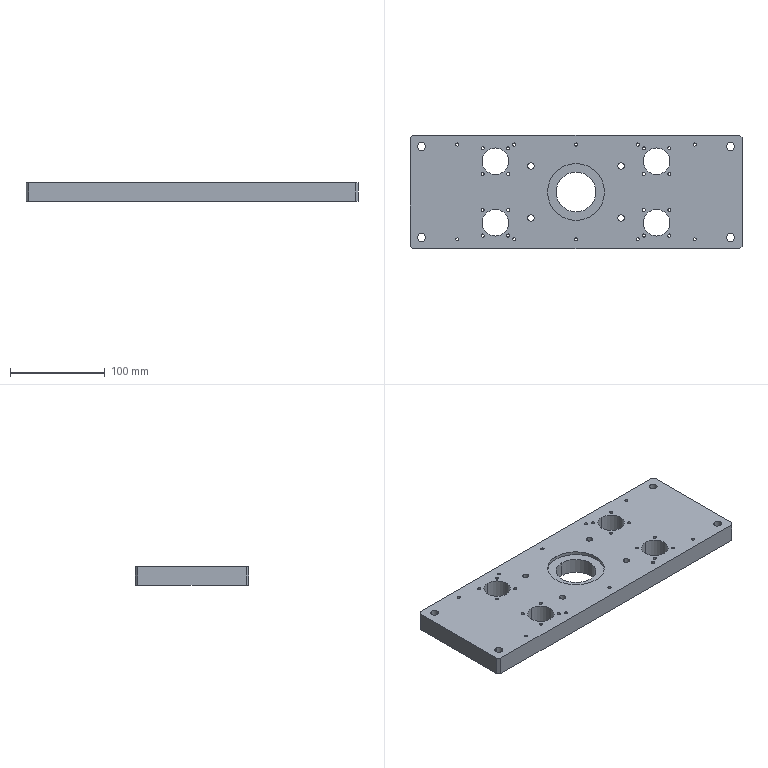Part | 1 solid | 103 faces | box 350 x 120 x 20 mm | volume 742845 mm3 | cylinder 88 | plane 15 | commonest cylinder face diameters 3.3 x52 6.8 x8 8.5 x8 16 x8 28 x8 42 x2